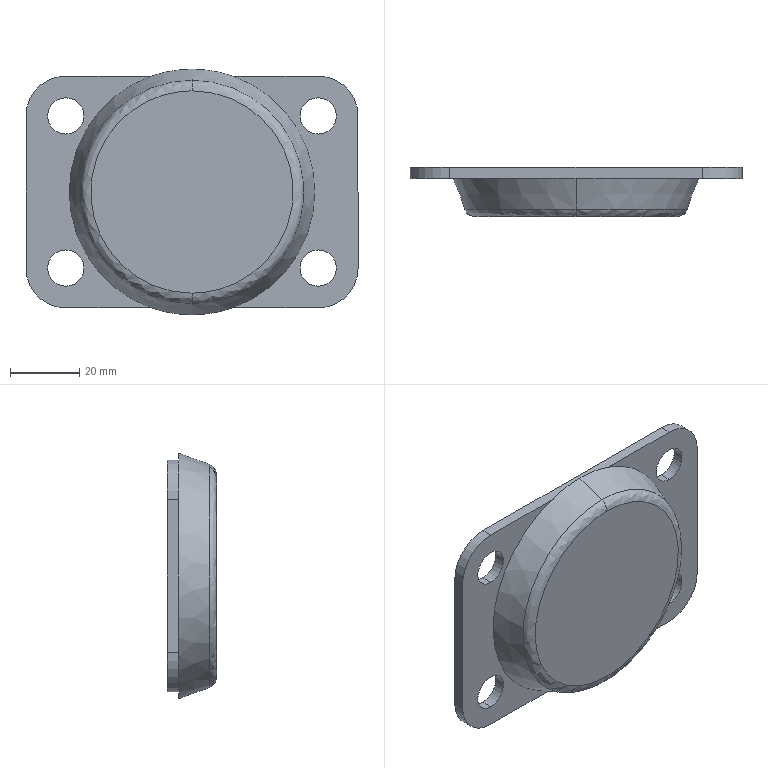Part | SolidWorks | features BaseBody 1 | 1 solid | 32 faces | box 96 x 14.2 x 71 mm | volume 54895 mm3 | cylinder 16 | plane 12 | spline 2 | cone 2 | commonest cylinder face diameters 10.5 x8 23 x4 27 x2 54 x2
STEP:
#1=CARTESIAN_POINT('',(0.,-12.094,-32.263));
#2=VERTEX_POINT('',#1);
#3=CARTESIAN_POINT('',(0.,-12.094,32.263));
#4=VERTEX_POINT('',#3);
#5=CARTESIAN_POINT('',(0.,-12.094,0.));
#6=DIRECTION('',(0.,1.,0.));
#7=DIRECTION('',(0.,0.,1.));
#8=AXIS2_PLACEMENT_3D('',#5,#6,#7);
#9=CIRCLE('',#8,32.263);
#10=EDGE_CURVE('',#2,#4,#9,.T.);
#11=ORIENTED_EDGE('',*,*,#10,.F.);
#12=CARTESIAN_POINT('',(0.,-14.2,-29.256));
#13=VERTEX_POINT('',#12);
#14=CARTESIAN_POINT('',(0.,-11.,-29.256));
#15=DIRECTION('',(-1.,0.,0.));
#16=DIRECTION('',(0.,0.,-1.));
#17=AXIS2_PLACEMENT_3D('',#14,#15,#16);
#18=CIRCLE('',#17,3.2);
#19=EDGE_CURVE('',#2,#13,#18,.T.);
#20=ORIENTED_EDGE('',*,*,#19,.T.);
#21=CARTESIAN_POINT('',(0.,-14.2,29.256));
#22=VERTEX_POINT('',#21);
#23=CARTESIAN_POINT('',(0.,-14.2,-29.256));
#24=CARTESIAN_POINT('',(-58.511,-14.2,-29.256));
#25=CARTESIAN_POINT('',(-58.511,-14.2,29.256));
#26=CARTESIAN_POINT('',(0.,-14.2,29.256));
#27=(BOUNDED_CURVE()B_SPLINE_CURVE(3,(#23,#24,#25,#26),.UNSPECIFIED.,.F.,.T.)B_SPLINE_CURVE_WITH_KNOTS((4,4),(0.,1.),.UNSPECIFIED.)CURVE()GEOMETRIC_REPRESENTATION_ITEM()RATIONAL_B_SPLINE_CURVE((1.,0.3333,0.3333,1.))REPRESENTATION_ITEM(''));
#28=EDGE_CURVE('',#13,#22,#27,.T.);
#29=ORIENTED_EDGE('',*,*,#28,.T.);
#30=CARTESIAN_POINT('',(0.,-11.,29.256));
#31=DIRECTION('',(1.,0.,0.));
#32=DIRECTION('',(0.,0.,1.));
#33=AXIS2_PLACEMENT_3D('',#30,#31,#32);
#34=CIRCLE('',#33,3.2);
#35=EDGE_CURVE('',#4,#22,#34,.T.);
#36=ORIENTED_EDGE('',*,*,#35,.F.);
#37=EDGE_LOOP('',(#11,#20,#29,#36));
#38=FACE_OUTER_BOUND('',#37,.T.);
#39=CARTESIAN_POINT('',(0.,-12.094,-32.263));
#40=CARTESIAN_POINT('',(-64.525,-12.094,-32.263));
#41=CARTESIAN_POINT('',(-64.525,-12.094,32.263));
#42=CARTESIAN_POINT('',(0.,-12.094,32.263));
#43=CARTESIAN_POINT('',(0.,-13.402,-31.787));
#44=CARTESIAN_POINT('',(-63.574,-13.402,-31.787));
#45=CARTESIAN_POINT('',(-63.574,-13.402,31.787));
#46=CARTESIAN_POINT('',(0.,-13.402,31.787));
#47=CARTESIAN_POINT('',(0.,-14.2,-30.647));
#48=CARTESIAN_POINT('',(-61.294,-14.2,-30.647));
#49=CARTESIAN_POINT('',(-61.294,-14.2,30.647));
#50=CARTESIAN_POINT('',(0.,-14.2,30.647));
#51=CARTESIAN_POINT('',(0.,-14.2,-29.256));
#52=CARTESIAN_POINT('',(-58.511,-14.2,-29.256));
#53=CARTESIAN_POINT('',(-58.511,-14.2,29.256));
#54=CARTESIAN_POINT('',(0.,-14.2,29.256));
#55=(BOUNDED_SURFACE()B_SPLINE_SURFACE(3,3,((#39,#40,#41,#42),(#43,#44,#45,#46),(#47,#48,#49,#50),(#51,#52,#53,#54)),.UNSPECIFIED.,.F.,.F.,.F.)B_SPLINE_SURFACE_WITH_KNOTS((4,4),(4,4),(0.,1.),(0.,1.),.UNSPECIFIED.)GEOMETRIC_REPRESENTATION_ITEM()RATIONAL_B_SPLINE_SURFACE(((1.,0.3333,0.3333,1.),(0.8794,0.2931,0.2931,0.8794),(0.8794,0.2931,0.2931,0.8794),(1.,0.3333,0.3333,1.)))REPRESENTATION_ITEM('')SURFACE());
#56=ADVANCED_FACE('',(#38),#55,.T.);
#57=CARTESIAN_POINT('',(36.5,-3.2,16.75));
#58=VERTEX_POINT('',#57);
#59=CARTESIAN_POINT('',(36.5,-3.2,27.25));
#60=VERTEX_POINT('',#59);
#61=CARTESIAN_POINT('',(36.5,-3.2,22.));
#62=DIRECTION('',(0.,1.,0.));
#63=DIRECTION('',(0.,0.,1.));
#64=AXIS2_PLACEMENT_3D('',#61,#62,#63);
#65=CIRCLE('',#64,5.25);
#66=EDGE_CURVE('',#58,#60,#65,.T.);
#67=ORIENTED_EDGE('',*,*,#66,.F.);
#68=CARTESIAN_POINT('',(36.5,0.,16.75));
#69=VERTEX_POINT('',#68);
#70=CARTESIAN_POINT('',(36.5,-3.2,16.75));
#71=DIRECTION('',(0.,1.,0.));
#72=VECTOR('',#71,1000.);
#73=LINE('',#70,#72);
#74=EDGE_CURVE('',#58,#69,#73,.T.);
#75=ORIENTED_EDGE('',*,*,#74,.T.);
#76=CARTESIAN_POINT('',(36.5,0.,27.25));
#77=VERTEX_POINT('',#76);
#78=CARTESIAN_POINT('',(36.5,0.,22.));
#79=DIRECTION('',(0.,-1.,0.));
#80=DIRECTION('',(0.,0.,1.));
#81=AXIS2_PLACEMENT_3D('',#78,#79,#80);
#82=CIRCLE('',#81,5.25);
#83=EDGE_CURVE('',#77,#69,#82,.T.);
#84=ORIENTED_EDGE('',*,*,#83,.F.);
#85=CARTESIAN_POINT('',(36.5,-3.2,27.25));
#86=DIRECTION('',(0.,1.,0.));
#87=VECTOR('',#86,1000.);
#88=LINE('',#85,#87);
#89=EDGE_CURVE('',#60,#77,#88,.T.);
#90=ORIENTED_EDGE('',*,*,#89,.F.);
#91=EDGE_LOOP('',(#67,#75,#84,#90));
#92=FACE_OUTER_BOUND('',#91,.T.);
#93=CARTESIAN_POINT('',(36.5,-3.2,22.));
#94=DIRECTION('',(0.,1.,0.));
#95=DIRECTION('',(0.,0.,1.));
#96=AXIS2_PLACEMENT_3D('',#93,#94,#95);
#97=CYLINDRICAL_SURFACE('',#96,5.25);
#98=ADVANCED_FACE('',(#92),#97,.F.);
#99=CARTESIAN_POINT('',(36.5,-3.2,-27.25));
#100=VERTEX_POINT('',#99);
#101=CARTESIAN_POINT('',(36.5,-3.2,-16.75));
#102=VERTEX_POINT('',#101);
#103=CARTESIAN_POINT('',(36.5,-3.2,-22.));
#104=DIRECTION('',(0.,1.,0.));
#105=DIRECTION('',(0.,0.,1.));
#106=AXIS2_PLACEMENT_3D('',#103,#104,#105);
#107=CIRCLE('',#106,5.25);
#108=EDGE_CURVE('',#100,#102,#107,.T.);
#109=ORIENTED_EDGE('',*,*,#108,.F.);
#110=CARTESIAN_POINT('',(36.5,0.,-27.25));
#111=VERTEX_POINT('',#110);
#112=CARTESIAN_POINT('',(36.5,-3.2,-27.25));
#113=DIRECTION('',(0.,1.,0.));
#114=VECTOR('',#113,1000.);
#115=LINE('',#112,#114);
#116=EDGE_CURVE('',#100,#111,#115,.T.);
#117=ORIENTED_EDGE('',*,*,#116,.T.);
#118=CARTESIAN_POINT('',(36.5,0.,-16.75));
#119=VERTEX_POINT('',#118);
#120=CARTESIAN_POINT('',(36.5,0.,-22.));
#121=DIRECTION('',(0.,-1.,0.));
#122=DIRECTION('',(0.,0.,1.));
#123=AXIS2_PLACEMENT_3D('',#120,#121,#122);
#124=CIRCLE('',#123,5.25);
#125=EDGE_CURVE('',#119,#111,#124,.T.);
#126=ORIENTED_EDGE('',*,*,#125,.F.);
#127=CARTESIAN_POINT('',(36.5,-3.2,-16.75));
#128=DIRECTION('',(0.,1.,0.));
#129=VECTOR('',#128,1000.);
#130=LINE('',#127,#129);
#131=EDGE_CURVE('',#102,#119,#130,.T.);
#132=ORIENTED_EDGE('',*,*,#131,.F.);
#133=EDGE_LOOP('',(#109,#117,#126,#132));
#134=FACE_OUTER_BOUND('',#133,.T.);
#135=CARTESIAN_POINT('',(36.5,-3.2,-22.));
#136=DIRECTION('',(0.,1.,0.));
#137=DIRECTION('',(0.,0.,1.));
#138=AXIS2_PLACEMENT_3D('',#135,#136,#137);
#139=CYLINDRICAL_SURFACE('',#138,5.25);
#140=ADVANCED_FACE('',(#134),#139,.F.);
#141=CARTESIAN_POINT('',(-36.5,-3.2,16.75));
#142=VERTEX_POINT('',#141);
#143=CARTESIAN_POINT('',(-36.5,-3.2,27.25));
#144=VERTEX_POINT('',#143);
#145=CARTESIAN_POINT('',(-36.5,-3.2,22.));
#146=DIRECTION('',(0.,1.,0.));
#147=DIRECTION('',(0.,0.,1.));
#148=AXIS2_PLACEMENT_3D('',#145,#146,#147);
#149=CIRCLE('',#148,5.25);
#150=EDGE_CURVE('',#142,#144,#149,.T.);
#151=ORIENTED_EDGE('',*,*,#150,.F.);
#152=CARTESIAN_POINT('',(-36.5,0.,16.75));
#153=VERTEX_POINT('',#152);
#154=CARTESIAN_POINT('',(-36.5,-3.2,16.75));
#155=DIRECTION('',(0.,1.,0.));
#156=VECTOR('',#155,1000.);
#157=LINE('',#154,#156);
#158=EDGE_CURVE('',#142,#153,#157,.T.);
#159=ORIENTED_EDGE('',*,*,#158,.T.);
#160=CARTESIAN_POINT('',(-36.5,0.,27.25));
#161=VERTEX_POINT('',#160);
#162=CARTESIAN_POINT('',(-36.5,0.,22.));
#163=DIRECTION('',(0.,-1.,0.));
#164=DIRECTION('',(0.,0.,1.));
#165=AXIS2_PLACEMENT_3D('',#162,#163,#164);
#166=CIRCLE('',#165,5.25);
#167=EDGE_CURVE('',#161,#153,#166,.T.);
#168=ORIENTED_EDGE('',*,*,#167,.F.);
#169=CARTESIAN_POINT('',(-36.5,-3.2,27.25));
#170=DIRECTION('',(0.,1.,0.));
#171=VECTOR('',#170,1000.);
#172=LINE('',#169,#171);
#173=EDGE_CURVE('',#144,#161,#172,.T.);
#174=ORIENTED_EDGE('',*,*,#173,.F.);
#175=EDGE_LOOP('',(#151,#159,#168,#174));
#176=FACE_OUTER_BOUND('',#175,.T.);
#177=CARTESIAN_POINT('',(-36.5,-3.2,22.));
#178=DIRECTION('',(0.,1.,0.));
#179=DIRECTION('',(0.,0.,1.));
#180=AXIS2_PLACEMENT_3D('',#177,#178,#179);
#181=CYLINDRICAL_SURFACE('',#180,5.25);
#182=ADVANCED_FACE('',(#176),#181,.F.);
#183=CARTESIAN_POINT('',(-36.5,-3.2,-27.25));
#184=VERTEX_POINT('',#183);
#185=CARTESIAN_POINT('',(-36.5,-3.2,-16.75));
#186=VERTEX_POINT('',#185);
#187=CARTESIAN_POINT('',(-36.5,-3.2,-22.));
#188=DIRECTION('',(0.,1.,0.));
#189=DIRECTION('',(0.,0.,1.));
#190=AXIS2_PLACEMENT_3D('',#187,#188,#189);
#191=CIRCLE('',#190,5.25);
#192=EDGE_CURVE('',#184,#186,#191,.T.);
#193=ORIENTED_EDGE('',*,*,#192,.F.);
#194=CARTESIAN_POINT('',(-36.5,0.,-27.25));
#195=VERTEX_POINT('',#194);
#196=CARTESIAN_POINT('',(-36.5,-3.2,-27.25));
#197=DIRECTION('',(0.,1.,0.));
#198=VECTOR('',#197,1000.);
#199=LINE('',#196,#198);
#200=EDGE_CURVE('',#184,#195,#199,.T.);
#201=ORIENTED_EDGE('',*,*,#200,.T.);
#202=CARTESIAN_POINT('',(-36.5,0.,-16.75));
#203=VERTEX_POINT('',#202);
#204=CARTESIAN_POINT('',(-36.5,0.,-22.));
#205=DIRECTION('',(0.,-1.,0.));
#206=DIRECTION('',(0.,0.,1.));
#207=AXIS2_PLACEMENT_3D('',#204,#205,#206);
#208=CIRCLE('',#207,5.25);
#209=EDGE_CURVE('',#203,#195,#208,.T.);
#210=ORIENTED_EDGE('',*,*,#209,.F.);
#211=CARTESIAN_POINT('',(-36.5,-3.2,-16.75));
#212=DIRECTION('',(0.,1.,0.));
#213=VECTOR('',#212,1000.);
#214=LINE('',#211,#213);
#215=EDGE_CURVE('',#186,#203,#214,.T.);
#216=ORIENTED_EDGE('',*,*,#215,.F.);
#217=EDGE_LOOP('',(#193,#201,#210,#216));
#218=FACE_OUTER_BOUND('',#217,.T.);
#219=CARTESIAN_POINT('',(-36.5,-3.2,-22.));
#220=DIRECTION('',(0.,1.,0.));
#221=DIRECTION('',(0.,0.,1.));
#222=AXIS2_PLACEMENT_3D('',#219,#220,#221);
#223=CYLINDRICAL_SURFACE('',#222,5.25);
#224=ADVANCED_FACE('',(#218),#223,.F.);
#225=CARTESIAN_POINT('',(0.,-1.5,-27.));
#226=VERTEX_POINT('',#225);
#227=CARTESIAN_POINT('',(0.,-1.5,27.));
#228=VERTEX_POINT('',#227);
#229=CARTESIAN_POINT('',(0.,-1.5,0.));
#230=DIRECTION('',(0.,1.,0.));
#231=DIRECTION('',(0.,0.,1.));
#232=AXIS2_PLACEMENT_3D('',#229,#230,#231);
#233=CIRCLE('',#232,27.);
#234=EDGE_CURVE('',#226,#228,#233,.T.);
#235=ORIENTED_EDGE('',*,*,#234,.F.);
#236=CARTESIAN_POINT('',(0.,0.,-27.));
#237=VERTEX_POINT('',#236);
#238=CARTESIAN_POINT('',(0.,-1.5,-27.));
#239=DIRECTION('',(0.,1.,0.));
#240=VECTOR('',#239,1000.);
#241=LINE('',#238,#240);
#242=EDGE_CURVE('',#226,#237,#241,.T.);
#243=ORIENTED_EDGE('',*,*,#242,.T.);
#244=CARTESIAN_POINT('',(0.,0.,27.));
#245=VERTEX_POINT('',#244);
#246=CARTESIAN_POINT('',(0.,0.,0.));
#247=DIRECTION('',(0.,-1.,0.));
#248=DIRECTION('',(0.,0.,1.));
#249=AXIS2_PLACEMENT_3D('',#246,#247,#248);
#250=CIRCLE('',#249,27.);
#251=EDGE_CURVE('',#245,#237,#250,.T.);
#252=ORIENTED_EDGE('',*,*,#251,.F.);
#253=CARTESIAN_POINT('',(0.,-1.5,27.));
#254=DIRECTION('',(0.,1.,0.));
#255=VECTOR('',#254,1000.);
#256=LINE('',#253,#255);
#257=EDGE_CURVE('',#228,#245,#256,.T.);
#258=ORIENTED_EDGE('',*,*,#257,.F.);
#259=EDGE_LOOP('',(#235,#243,#252,#258));
#260=FACE_OUTER_BOUND('',#259,.T.);
#261=CARTESIAN_POINT('',(0.,-1.5,0.));
#262=DIRECTION('',(0.,1.,0.));
#263=DIRECTION('',(0.,0.,1.));
#264=AXIS2_PLACEMENT_3D('',#261,#262,#263);
#265=CYLINDRICAL_SURFACE('',#264,27.);
#266=ADVANCED_FACE('',(#260),#265,.F.);
#267=CARTESIAN_POINT('',(0.,-12.094,0.));
#268=DIRECTION('',(0.,1.,0.));
#269=DIRECTION('',(0.,0.,1.));
#270=AXIS2_PLACEMENT_3D('',#267,#268,#269);
#271=CIRCLE('',#270,32.263);
#272=EDGE_CURVE('',#4,#2,#271,.T.);
#273=ORIENTED_EDGE('',*,*,#272,.T.);
#274=CARTESIAN_POINT('',(0.,-3.2,-35.5));
#275=VERTEX_POINT('',#274);
#276=CARTESIAN_POINT('',(0.,-3.2,-35.5));
#277=DIRECTION('',(0.,0.9397,-0.342));
#278=VECTOR('',#277,1000.);
#279=LINE('',#276,#278);
#280=EDGE_CURVE('',#2,#275,#279,.T.);
#281=ORIENTED_EDGE('',*,*,#280,.T.);
#282=CARTESIAN_POINT('',(11.747,-3.2,-33.5));
#283=VERTEX_POINT('',#282);
#284=CARTESIAN_POINT('',(0.,-3.2,0.));
#285=DIRECTION('',(0.,1.,0.));
#286=DIRECTION('',(0.,0.,1.));
#287=AXIS2_PLACEMENT_3D('',#284,#285,#286);
#288=CIRCLE('',#287,35.5);
#289=EDGE_CURVE('',#283,#275,#288,.T.);
#290=ORIENTED_EDGE('',*,*,#289,.F.);
#291=CARTESIAN_POINT('',(11.747,-3.2,33.5));
#292=VERTEX_POINT('',#291);
#293=CARTESIAN_POINT('',(0.,-3.2,0.));
#294=DIRECTION('',(0.,-1.,0.));
#295=DIRECTION('',(0.,0.,1.));
#296=AXIS2_PLACEMENT_3D('',#293,#294,#295);
#297=CIRCLE('',#296,35.5);
#298=EDGE_CURVE('',#283,#292,#297,.T.);
#299=ORIENTED_EDGE('',*,*,#298,.T.);
#300=CARTESIAN_POINT('',(0.,-3.2,35.5));
#301=VERTEX_POINT('',#300);
#302=CARTESIAN_POINT('',(0.,-3.2,0.));
#303=DIRECTION('',(0.,1.,0.));
#304=DIRECTION('',(0.,0.,1.));
#305=AXIS2_PLACEMENT_3D('',#302,#303,#304);
#306=CIRCLE('',#305,35.5);
#307=EDGE_CURVE('',#301,#292,#306,.T.);
#308=ORIENTED_EDGE('',*,*,#307,.F.);
#309=CARTESIAN_POINT('',(0.,-3.2,35.5));
#310=DIRECTION('',(0.,0.9397,0.342));
#311=VECTOR('',#310,1000.);
#312=LINE('',#309,#311);
#313=EDGE_CURVE('',#4,#301,#312,.T.);
#314=ORIENTED_EDGE('',*,*,#313,.F.);
#315=EDGE_LOOP('',(#273,#281,#290,#299,#308,#314));
#316=FACE_OUTER_BOUND('',#315,.T.);
#317=CARTESIAN_POINT('',(0.,-3.2,0.));
#318=DIRECTION('',(0.,1.,0.));
#319=DIRECTION('',(0.,0.,1.));
#320=AXIS2_PLACEMENT_3D('',#317,#318,#319);
#321=CONICAL_SURFACE('',#320,35.5,0.3491);
#322=ADVANCED_FACE('',(#316),#321,.T.);
#323=CARTESIAN_POINT('',(0.,-0.5,-13.5));
#324=VERTEX_POINT('',#323);
#325=CARTESIAN_POINT('',(0.,-0.5,13.5));
#326=VERTEX_POINT('',#325);
#327=CARTESIAN_POINT('',(0.,-0.5,0.));
#328=DIRECTION('',(0.,-1.,0.));
#329=DIRECTION('',(0.,0.,-1.));
#330=AXIS2_PLACEMENT_3D('',#327,#328,#329);
#331=CIRCLE('',#330,13.5);
#332=EDGE_CURVE('',#324,#326,#331,.T.);
#333=ORIENTED_EDGE('',*,*,#332,.T.);
#334=CARTESIAN_POINT('',(0.,-1.5,13.5));
#335=VERTEX_POINT('',#334);
#336=CARTESIAN_POINT('',(0.,-0.5,13.5));
#337=DIRECTION('',(0.,-1.,0.));
#338=VECTOR('',#337,1000.);
#339=LINE('',#336,#338);
#340=EDGE_CURVE('',#326,#335,#339,.T.);
#341=ORIENTED_EDGE('',*,*,#340,.T.);
#342=CARTESIAN_POINT('',(0.,-1.5,-13.5));
#343=VERTEX_POINT('',#342);
#344=CARTESIAN_POINT('',(0.,-1.5,0.));
#345=DIRECTION('',(0.,-1.,0.));
#346=DIRECTION('',(0.,0.,-1.));
#347=AXIS2_PLACEMENT_3D('',#344,#345,#346);
#348=CIRCLE('',#347,13.5);
#349=EDGE_CURVE('',#343,#335,#348,.T.);
#350=ORIENTED_EDGE('',*,*,#349,.F.);
#351=CARTESIAN_POINT('',(0.,-0.5,-13.5));
#352=DIRECTION('',(0.,-1.,0.));
#353=VECTOR('',#352,1000.);
#354=LINE('',#351,#353);
#355=EDGE_CURVE('',#324,#343,#354,.T.);
#356=ORIENTED_EDGE('',*,*,#355,.F.);
#357=EDGE_LOOP('',(#333,#341,#350,#356));
#358=FACE_OUTER_BOUND('',#357,.T.);
#359=CARTESIAN_POINT('',(0.,-0.5,0.));
#360=DIRECTION('',(0.,-1.,0.));
#361=DIRECTION('',(0.,0.,-1.));
#362=AXIS2_PLACEMENT_3D('',#359,#360,#361);
#363=CYLINDRICAL_SURFACE('',#362,13.5);
#364=ADVANCED_FACE('',(#358),#363,.T.);
#365=CARTESIAN_POINT('',(-36.5,0.,-33.5));
#366=VERTEX_POINT('',#365);
#367=CARTESIAN_POINT('',(-48.,0.,-22.));
#368=VERTEX_POINT('',#367);
#369=CARTESIAN_POINT('',(-36.5,0.,-22.));
#370=DIRECTION('',(0.,1.,0.));
#371=DIRECTION('',(0.,0.,1.));
#372=AXIS2_PLACEMENT_3D('',#369,#370,#371);
#373=CIRCLE('',#372,11.5);
#374=EDGE_CURVE('',#366,#368,#373,.T.);
#375=ORIENTED_EDGE('',*,*,#374,.T.);
#376=CARTESIAN_POINT('',(-48.,0.,22.));
#377=VERTEX_POINT('',#376);
#378=CARTESIAN_POINT('',(-48.,0.,22.));
#379=DIRECTION('',(0.,0.,1.));
#380=VECTOR('',#379,1000.);
#381=LINE('',#378,#380);
#382=EDGE_CURVE('',#368,#377,#381,.T.);
#383=ORIENTED_EDGE('',*,*,#382,.T.);
#384=CARTESIAN_POINT('',(-36.5,0.,33.5));
#385=VERTEX_POINT('',#384);
#386=CARTESIAN_POINT('',(-36.5,0.,22.));
#387=DIRECTION('',(0.,1.,0.));
#388=DIRECTION('',(0.,0.,1.));
#389=AXIS2_PLACEMENT_3D('',#386,#387,#388);
#390=CIRCLE('',#389,11.5);
#391=EDGE_CURVE('',#377,#385,#390,.T.);
#392=ORIENTED_EDGE('',*,*,#391,.T.);
#393=CARTESIAN_POINT('',(36.5,0.,33.5));
#394=VERTEX_POINT('',#393);
#395=CARTESIAN_POINT('',(-36.5,0.,33.5));
#396=DIRECTION('',(1.,0.,0.));
#397=VECTOR('',#396,1000.);
#398=LINE('',#395,#397);
#399=EDGE_CURVE('',#385,#394,#398,.T.);
#400=ORIENTED_EDGE('',*,*,#399,.T.);
#401=CARTESIAN_POINT('',(48.,0.,22.));
#402=VERTEX_POINT('',#401);
#403=CARTESIAN_POINT('',(36.5,0.,22.));
#404=DIRECTION('',(0.,1.,0.));
#405=DIRECTION('',(0.,0.,1.));
#406=AXIS2_PLACEMENT_3D('',#403,#404,#405);
#407=CIRCLE('',#406,11.5);
#408=EDGE_CURVE('',#394,#402,#407,.T.);
#409=ORIENTED_EDGE('',*,*,#408,.T.);
#410=CARTESIAN_POINT('',(48.,0.,-22.));
#411=VERTEX_POINT('',#410);
#412=CARTESIAN_POINT('',(48.,0.,22.));
#413=DIRECTION('',(0.,0.,-1.));
#414=VECTOR('',#413,1000.);
#415=LINE('',#412,#414);
#416=EDGE_CURVE('',#402,#411,#415,.T.);
#417=ORIENTED_EDGE('',*,*,#416,.T.);
#418=CARTESIAN_POINT('',(36.5,0.,-33.5));
#419=VERTEX_POINT('',#418);
#420=CARTESIAN_POINT('',(36.5,0.,-22.));
#421=DIRECTION('',(0.,1.,0.));
#422=DIRECTION('',(0.,0.,1.));
#423=AXIS2_PLACEMENT_3D('',#420,#421,#422);
#424=CIRCLE('',#423,11.5);
#425=EDGE_CURVE('',#411,#419,#424,.T.);
#426=ORIENTED_EDGE('',*,*,#425,.T.);
#427=CARTESIAN_POINT('',(-36.5,0.,-33.5));
#428=DIRECTION('',(-1.,0.,0.));
#429=VECTOR('',#428,1000.);
#430=LINE('',#427,#429);
#431=EDGE_CURVE('',#419,#366,#430,.T.);
#432=ORIENTED_EDGE('',*,*,#431,.T.);
#433=EDGE_LOOP('',(#375,#383,#392,#400,#409,#417,#426,#432));
#434=FACE_OUTER_BOUND('',#433,.T.);
#435=ORIENTED_EDGE('',*,*,#83,.T.);
#436=CARTESIAN_POINT('',(36.5,0.,22.));
#437=DIRECTION('',(0.,-1.,0.));
#438=DIRECTION('',(0.,0.,1.));
#439=AXIS2_PLACEMENT_3D('',#436,#437,#438);
#440=CIRCLE('',#439,5.25);
#441=EDGE_CURVE('',#69,#77,#440,.T.);
#442=ORIENTED_EDGE('',*,*,#441,.T.);
#443=EDGE_LOOP('',(#435,#442));
#444=FACE_BOUND('',#443,.T.);
#445=ORIENTED_EDGE('',*,*,#125,.T.);
#446=CARTESIAN_POINT('',(36.5,0.,-22.));
#447=DIRECTION('',(0.,-1.,0.));
#448=DIRECTION('',(0.,0.,1.));
#449=AXIS2_PLACEMENT_3D('',#446,#447,#448);
#450=CIRCLE('',#449,5.25);
#451=EDGE_CURVE('',#111,#119,#450,.T.);
#452=ORIENTED_EDGE('',*,*,#451,.T.);
#453=EDGE_LOOP('',(#445,#452));
#454=FACE_BOUND('',#453,.T.);
#455=ORIENTED_EDGE('',*,*,#167,.T.);
#456=CARTESIAN_POINT('',(-36.5,0.,22.));
#457=DIRECTION('',(0.,-1.,0.));
#458=DIRECTION('',(0.,0.,1.));
#459=AXIS2_PLACEMENT_3D('',#456,#457,#458);
#460=CIRCLE('',#459,5.25);
#461=EDGE_CURVE('',#153,#161,#460,.T.);
#462=ORIENTED_EDGE('',*,*,#461,.T.);
#463=EDGE_LOOP('',(#455,#462));
#464=FACE_BOUND('',#463,.T.);
#465=ORIENTED_EDGE('',*,*,#209,.T.);
#466=CARTESIAN_POINT('',(-36.5,0.,-22.));
#467=DIRECTION('',(0.,-1.,0.));
#468=DIRECTION('',(0.,0.,1.));
#469=AXIS2_PLACEMENT_3D('',#466,#467,#468);
#470=CIRCLE('',#469,5.25);
#471=EDGE_CURVE('',#195,#203,#470,.T.);
#472=ORIENTED_EDGE('',*,*,#471,.T.);
#473=EDGE_LOOP('',(#465,#472));
#474=FACE_BOUND('',#473,.T.);
#475=ORIENTED_EDGE('',*,*,#251,.T.);
#476=CARTESIAN_POINT('',(0.,0.,0.));
#477=DIRECTION('',(0.,-1.,0.));
#478=DIRECTION('',(0.,0.,1.));
#479=AXIS2_PLACEMENT_3D('',#476,#477,#478);
#480=CIRCLE('',#479,27.);
#481=EDGE_CURVE('',#237,#245,#480,.T.);
#482=ORIENTED_EDGE('',*,*,#481,.T.);
#483=EDGE_LOOP('',(#475,#482));
#484=FACE_BOUND('',#483,.T.);
#485=CARTESIAN_POINT('',(-36.5,0.,22.));
#486=DIRECTION('',(0.,1.,0.));
#487=DIRECTION('',(0.,0.,1.));
#488=AXIS2_PLACEMENT_3D('',#485,#486,#487);
#489=PLANE('',#488);
#490=ADVANCED_FACE('',(#434,#444,#454,#464,#474,#484),#489,.T.);
#491=CARTESIAN_POINT('',(-48.,-3.2,-22.));
#492=VERTEX_POINT('',#491);
#493=CARTESIAN_POINT('',(-48.,-3.2,22.));
#494=VERTEX_POINT('',#493);
#495=CARTESIAN_POINT('',(-48.,-3.2,-22.));
#496=DIRECTION('',(0.,0.,1.));
#497=VECTOR('',#496,1000.);
#498=LINE('',#495,#497);
#499=EDGE_CURVE('',#492,#494,#498,.T.);
#500=ORIENTED_EDGE('',*,*,#499,.T.);
#501=CARTESIAN_POINT('',(-48.,-3.2,22.));
#502=DIRECTION('',(0.,1.,0.));
#503=VECTOR('',#502,1000.);
#504=LINE('',#501,#503);
#505=EDGE_CURVE('',#494,#377,#504,.T.);
#506=ORIENTED_EDGE('',*,*,#505,.T.);
#507=ORIENTED_EDGE('',*,*,#382,.F.);
#508=CARTESIAN_POINT('',(-48.,-3.2,-22.));
#509=DIRECTION('',(0.,-1.,0.));
#510=VECTOR('',#509,1000.);
#511=LINE('',#508,#510);
#512=EDGE_CURVE('',#368,#492,#511,.T.);
#513=ORIENTED_EDGE('',*,*,#512,.T.);
#514=EDGE_LOOP('',(#500,#506,#507,#513));
#515=FACE_OUTER_BOUND('',#514,.T.);
#516=CARTESIAN_POINT('',(-48.,-3.2,-22.));
#517=DIRECTION('',(-1.,0.,0.));
#518=DIRECTION('',(0.,0.,1.));
#519=AXIS2_PLACEMENT_3D('',#516,#517,#518);
#520=PLANE('',#519);
#521=ADVANCED_FACE('',(#515),#520,.T.);
#522=CARTESIAN_POINT('',(-36.5,-3.2,-33.5));
#523=VERTEX_POINT('',#522);
#524=CARTESIAN_POINT('',(-36.5,-3.2,-22.));
#525=DIRECTION('',(0.,1.,0.));
#526=DIRECTION('',(0.,0.,1.));
#527=AXIS2_PLACEMENT_3D('',#524,#525,#526);
#528=CIRCLE('',#527,11.5);
#529=EDGE_CURVE('',#523,#492,#528,.T.);
#530=ORIENTED_EDGE('',*,*,#529,.T.);
#531=ORIENTED_EDGE('',*,*,#512,.F.);
#532=ORIENTED_EDGE('',*,*,#374,.F.);
#533=CARTESIAN_POINT('',(-36.5,-3.2,-33.5));
#534=DIRECTION('',(0.,-1.,0.));
#535=VECTOR('',#534,1000.);
#536=LINE('',#533,#535);
#537=EDGE_CURVE('',#366,#523,#536,.T.);
#538=ORIENTED_EDGE('',*,*,#537,.T.);
#539=EDGE_LOOP('',(#530,#531,#532,#538));
#540=FACE_OUTER_BOUND('',#539,.T.);
#541=CARTESIAN_POINT('',(-36.5,-3.2,-22.));
#542=DIRECTION('',(0.,1.,0.));
#543=DIRECTION('',(0.,0.,1.));
#544=AXIS2_PLACEMENT_3D('',#541,#542,#543);
#545=CYLINDRICAL_SURFACE('',#544,11.5);
#546=ADVANCED_FACE('',(#540),#545,.T.);
#547=CARTESIAN_POINT('',(-11.747,-3.2,-33.5));
#548=VERTEX_POINT('',#547);
#549=CARTESIAN_POINT('',(36.5,-3.2,-33.5));
#550=DIRECTION('',(-1.,0.,0.));
#551=VECTOR('',#550,1000.);
#552=LINE('',#549,#551);
#553=EDGE_CURVE('',#548,#523,#552,.T.);
#554=ORIENTED_EDGE('',*,*,#553,.T.);
#555=ORIENTED_EDGE('',*,*,#537,.F.);
#556=ORIENTED_EDGE('',*,*,#431,.F.);
#557=CARTESIAN_POINT('',(36.5,-3.2,-33.5));
#558=VERTEX_POINT('',#557);
#559=CARTESIAN_POINT('',(36.5,-3.2,-33.5));
#560=DIRECTION('',(0.,-1.,0.));
#561=VECTOR('',#560,1000.);
#562=LINE('',#559,#561);
#563=EDGE_CURVE('',#419,#558,#562,.T.);
#564=ORIENTED_EDGE('',*,*,#563,.T.);
#565=CARTESIAN_POINT('',(36.5,-3.2,-33.5));
#566=DIRECTION('',(-1.,0.,0.));
#567=VECTOR('',#566,1000.);
#568=LINE('',#565,#567);
#569=EDGE_CURVE('',#558,#283,#568,.T.);
#570=ORIENTED_EDGE('',*,*,#569,.T.);
#571=CARTESIAN_POINT('',(36.5,-3.2,-33.5));
#572=DIRECTION('',(-1.,0.,0.));
#573=VECTOR('',#572,1000.);
#574=LINE('',#571,#573);
#575=EDGE_CURVE('',#283,#548,#574,.T.);
#576=ORIENTED_EDGE('',*,*,#575,.T.);
#577=EDGE_LOOP('',(#554,#555,#556,#564,#570,#576));
#578=FACE_OUTER_BOUND('',#577,.T.);
#579=CARTESIAN_POINT('',(36.5,-3.2,-33.5));
#580=DIRECTION('',(0.,0.,-1.));
#581=DIRECTION('',(-1.,0.,0.));
#582=AXIS2_PLACEMENT_3D('',#579,#580,#581);
#583=PLANE('',#582);
#584=ADVANCED_FACE('',(#578),#583,.T.);
#585=CARTESIAN_POINT('',(48.,-3.2,-22.));
#586=VERTEX_POINT('',#585);
#587=CARTESIAN_POINT('',(36.5,-3.2,-22.));
#588=DIRECTION('',(0.,1.,0.));
#589=DIRECTION('',(0.,0.,1.));
#590=AXIS2_PLACEMENT_3D('',#587,#588,#589);
#591=CIRCLE('',#590,11.5);
#592=EDGE_CURVE('',#586,#558,#591,.T.);
#593=ORIENTED_EDGE('',*,*,#592,.T.);
#594=ORIENTED_EDGE('',*,*,#563,.F.);
#595=ORIENTED_EDGE('',*,*,#425,.F.);
#596=CARTESIAN_POINT('',(48.,-3.2,-22.));
#597=DIRECTION('',(0.,-1.,0.));
#598=VECTOR('',#597,1000.);
#599=LINE('',#596,#598);
#600=EDGE_CURVE('',#411,#586,#599,.T.);
#601=ORIENTED_EDGE('',*,*,#600,.T.);
#602=EDGE_LOOP('',(#593,#594,#595,#601));
#603=FACE_OUTER_BOUND('',#602,.T.);
#604=CARTESIAN_POINT('',(36.5,-3.2,-22.));
#605=DIRECTION('',(0.,1.,0.));
#606=DIRECTION('',(0.,0.,1.));
#607=AXIS2_PLACEMENT_3D('',#604,#605,#606);
#608=CYLINDRICAL_SURFACE('',#607,11.5);
#609=ADVANCED_FACE('',(#603),#608,.T.);
#610=CARTESIAN_POINT('',(48.,-3.2,22.));
#611=VERTEX_POINT('',#610);
#612=CARTESIAN_POINT('',(48.,-3.2,22.));
#613=DIRECTION('',(0.,0.,-1.));
#614=VECTOR('',#613,1000.);
#615=LINE('',#612,#614);
#616=EDGE_CURVE('',#611,#586,#615,.T.);
#617=ORIENTED_EDGE('',*,*,#616,.T.);
#618=ORIENTED_EDGE('',*,*,#600,.F.);
#619=ORIENTED_EDGE('',*,*,#416,.F.);
#620=CARTESIAN_POINT('',(48.,-3.2,22.));
#621=DIRECTION('',(0.,-1.,0.));
#622=VECTOR('',#621,1000.);
#623=LINE('',#620,#622);
#624=EDGE_CURVE('',#402,#611,#623,.T.);
#625=ORIENTED_EDGE('',*,*,#624,.T.);
#626=EDGE_LOOP('',(#617,#618,#619,#625));
#627=FACE_OUTER_BOUND('',#626,.T.);
#628=CARTESIAN_POINT('',(48.,-3.2,22.));
#629=DIRECTION('',(1.,0.,0.));
#630=DIRECTION('',(0.,0.,-1.));
#631=AXIS2_PLACEMENT_3D('',#628,#629,#630);
#632=PLANE('',#631);
#633=ADVANCED_FACE('',(#627),#632,.T.);
#634=CARTESIAN_POINT('',(36.5,-3.2,33.5));
#635=VERTEX_POINT('',#634);
#636=CARTESIAN_POINT('',(36.5,-3.2,22.));
#637=DIRECTION('',(0.,1.,0.));
#638=DIRECTION('',(0.,0.,1.));
#639=AXIS2_PLACEMENT_3D('',#636,#637,#638);
#640=CIRCLE('',#639,11.5);
#641=EDGE_CURVE('',#635,#611,#640,.T.);
#642=ORIENTED_EDGE('',*,*,#641,.T.);
#643=ORIENTED_EDGE('',*,*,#624,.F.);
#644=ORIENTED_EDGE('',*,*,#408,.F.);
#645=CARTESIAN_POINT('',(36.5,-3.2,33.5));
#646=DIRECTION('',(0.,-1.,0.));
#647=VECTOR('',#646,1000.);
#648=LINE('',#645,#647);
#649=EDGE_CURVE('',#394,#635,#648,.T.);
#650=ORIENTED_EDGE('',*,*,#649,.T.);
#651=EDGE_LOOP('',(#642,#643,#644,#650));
#652=FACE_OUTER_BOUND('',#651,.T.);
#653=CARTESIAN_POINT('',(36.5,-3.2,22.));
#654=DIRECTION('',(0.,1.,0.));
#655=DIRECTION('',(0.,0.,1.));
#656=AXIS2_PLACEMENT_3D('',#653,#654,#655);
#657=CYLINDRICAL_SURFACE('',#656,11.5);
#658=ADVANCED_FACE('',(#652),#657,.T.);
#659=CARTESIAN_POINT('',(-36.5,-3.2,33.5));
#660=DIRECTION('',(1.,0.,0.));
#661=VECTOR('',#660,1000.);
#662=LINE('',#659,#661);
#663=EDGE_CURVE('',#292,#635,#662,.T.);
#664=ORIENTED_EDGE('',*,*,#663,.T.);
#665=ORIENTED_EDGE('',*,*,#649,.F.);
#666=ORIENTED_EDGE('',*,*,#399,.F.);
#667=CARTESIAN_POINT('',(-36.5,-3.2,33.5));
#668=VERTEX_POINT('',#667);
#669=CARTESIAN_POINT('',(-36.5,-3.2,33.5));
#670=DIRECTION('',(0.,-1.,0.));
#671=VECTOR('',#670,1000.);
#672=LINE('',#669,#671);
#673=EDGE_CURVE('',#385,#668,#672,.T.);
#674=ORIENTED_EDGE('',*,*,#673,.T.);
#675=CARTESIAN_POINT('',(-11.747,-3.2,33.5));
#676=VERTEX_POINT('',#675);
#677=CARTESIAN_POINT('',(-36.5,-3.2,33.5));
#678=DIRECTION('',(1.,0.,0.));
#679=VECTOR('',#678,1000.);
#680=LINE('',#677,#679);
#681=EDGE_CURVE('',#668,#676,#680,.T.);
#682=ORIENTED_EDGE('',*,*,#681,.T.);
#683=CARTESIAN_POINT('',(-36.5,-3.2,33.5));
#684=DIRECTION('',(1.,0.,0.));
#685=VECTOR('',#684,1000.);
#686=LINE('',#683,#685);
#687=EDGE_CURVE('',#676,#292,#686,.T.);
#688=ORIENTED_EDGE('',*,*,#687,.T.);
#689=EDGE_LOOP('',(#664,#665,#666,#674,#682,#688));
#690=FACE_OUTER_BOUND('',#689,.T.);
#691=CARTESIAN_POINT('',(-36.5,-3.2,33.5));
#692=DIRECTION('',(0.,0.,1.));
#693=DIRECTION('',(1.,0.,0.));
#694=AXIS2_PLACEMENT_3D('',#691,#692,#693);
#695=PLANE('',#694);
#696=ADVANCED_FACE('',(#690),#695,.T.);
#697=CARTESIAN_POINT('',(-36.5,-3.2,22.));
#698=DIRECTION('',(0.,1.,0.));
#699=DIRECTION('',(0.,0.,1.));
#700=AXIS2_PLACEMENT_3D('',#697,#698,#699);
#701=CIRCLE('',#700,11.5);
#702=EDGE_CURVE('',#494,#668,#701,.T.);
#703=ORIENTED_EDGE('',*,*,#702,.T.);
#704=ORIENTED_EDGE('',*,*,#673,.F.);
#705=ORIENTED_EDGE('',*,*,#391,.F.);
#706=ORIENTED_EDGE('',*,*,#505,.F.);
#707=EDGE_LOOP('',(#703,#704,#705,#706));
#708=FACE_OUTER_BOUND('',#707,.T.);
#709=CARTESIAN_POINT('',(-36.5,-3.2,22.));
#710=DIRECTION('',(0.,1.,0.));
#711=DIRECTION('',(0.,0.,1.));
#712=AXIS2_PLACEMENT_3D('',#709,#710,#711);
#713=CYLINDRICAL_SURFACE('',#712,11.5);
#714=ADVANCED_FACE('',(#708),#713,.T.);
#715=ORIENTED_EDGE('',*,*,#74,.F.);
#716=CARTESIAN_POINT('',(36.5,-3.2,22.));
#717=DIRECTION('',(0.,1.,0.));
#718=DIRECTION('',(0.,0.,1.));
#719=AXIS2_PLACEMENT_3D('',#716,#717,#718);
#720=CIRCLE('',#719,5.25);
#721=EDGE_CURVE('',#60,#58,#720,.T.);
#722=ORIENTED_EDGE('',*,*,#721,.F.);
#723=ORIENTED_EDGE('',*,*,#89,.T.);
#724=ORIENTED_EDGE('',*,*,#441,.F.);
#725=EDGE_LOOP('',(#715,#722,#723,#724));
#726=FACE_OUTER_BOUND('',#725,.T.);
#727=CARTESIAN_POINT('',(36.5,-3.2,22.));
#728=DIRECTION('',(0.,1.,0.));
#729=DIRECTION('',(0.,0.,1.));
#730=AXIS2_PLACEMENT_3D('',#727,#728,#729);
#731=CYLINDRICAL_SURFACE('',#730,5.25);
#732=ADVANCED_FACE('',(#726),#731,.F.);
#733=ORIENTED_EDGE('',*,*,#116,.F.);
#734=CARTESIAN_POINT('',(36.5,-3.2,-22.));
#735=DIRECTION('',(0.,1.,0.));
#736=DIRECTION('',(0.,0.,1.));
#737=AXIS2_PLACEMENT_3D('',#734,#735,#736);
#738=CIRCLE('',#737,5.25);
#739=EDGE_CURVE('',#102,#100,#738,.T.);
#740=ORIENTED_EDGE('',*,*,#739,.F.);
#741=ORIENTED_EDGE('',*,*,#131,.T.);
#742=ORIENTED_EDGE('',*,*,#451,.F.);
#743=EDGE_LOOP('',(#733,#740,#741,#742));
#744=FACE_OUTER_BOUND('',#743,.T.);
#745=CARTESIAN_POINT('',(36.5,-3.2,-22.));
#746=DIRECTION('',(0.,1.,0.));
#747=DIRECTION('',(0.,0.,1.));
#748=AXIS2_PLACEMENT_3D('',#745,#746,#747);
#749=CYLINDRICAL_SURFACE('',#748,5.25);
#750=ADVANCED_FACE('',(#744),#749,.F.);
#751=ORIENTED_EDGE('',*,*,#158,.F.);
#752=CARTESIAN_POINT('',(-36.5,-3.2,22.));
#753=DIRECTION('',(0.,1.,0.));
#754=DIRECTION('',(0.,0.,1.));
#755=AXIS2_PLACEMENT_3D('',#752,#753,#754);
#756=CIRCLE('',#755,5.25);
#757=EDGE_CURVE('',#144,#142,#756,.T.);
#758=ORIENTED_EDGE('',*,*,#757,.F.);
#759=ORIENTED_EDGE('',*,*,#173,.T.);
#760=ORIENTED_EDGE('',*,*,#461,.F.);
#761=EDGE_LOOP('',(#751,#758,#759,#760));
#762=FACE_OUTER_BOUND('',#761,.T.);
#763=CARTESIAN_POINT('',(-36.5,-3.2,22.));
#764=DIRECTION('',(0.,1.,0.));
#765=DIRECTION('',(0.,0.,1.));
#766=AXIS2_PLACEMENT_3D('',#763,#764,#765);
#767=CYLINDRICAL_SURFACE('',#766,5.25);
#768=ADVANCED_FACE('',(#762),#767,.F.);
#769=ORIENTED_EDGE('',*,*,#200,.F.);
#770=CARTESIAN_POINT('',(-36.5,-3.2,-22.));
#771=DIRECTION('',(0.,1.,0.));
#772=DIRECTION('',(0.,0.,1.));
#773=AXIS2_PLACEMENT_3D('',#770,#771,#772);
#774=CIRCLE('',#773,5.25);
#775=EDGE_CURVE('',#186,#184,#774,.T.);
#776=ORIENTED_EDGE('',*,*,#775,.F.);
#777=ORIENTED_EDGE('',*,*,#215,.T.);
#778=ORIENTED_EDGE('',*,*,#471,.F.);
#779=EDGE_LOOP('',(#769,#776,#777,#778));
#780=FACE_OUTER_BOUND('',#779,.T.);
#781=CARTESIAN_POINT('',(-36.5,-3.2,-22.));
#782=DIRECTION('',(0.,1.,0.));
#783=DIRECTION('',(0.,0.,1.));
#784=AXIS2_PLACEMENT_3D('',#781,#782,#783);
#785=CYLINDRICAL_SURFACE('',#784,5.25);
#786=ADVANCED_FACE('',(#780),#785,.F.);
#787=ORIENTED_EDGE('',*,*,#242,.F.);
#788=CARTESIAN_POINT('',(0.,-1.5,0.));
#789=DIRECTION('',(0.,1.,0.));
#790=DIRECTION('',(0.,0.,1.));
#791=AXIS2_PLACEMENT_3D('',#788,#789,#790);
#792=CIRCLE('',#791,27.);
#793=EDGE_CURVE('',#228,#226,#792,.T.);
#794=ORIENTED_EDGE('',*,*,#793,.F.);
#795=ORIENTED_EDGE('',*,*,#257,.T.);
#796=ORIENTED_EDGE('',*,*,#481,.F.);
#797=EDGE_LOOP('',(#787,#794,#795,#796));
#798=FACE_OUTER_BOUND('',#797,.T.);
#799=CARTESIAN_POINT('',(0.,-1.5,0.));
#800=DIRECTION('',(0.,1.,0.));
#801=DIRECTION('',(0.,0.,1.));
#802=AXIS2_PLACEMENT_3D('',#799,#800,#801);
#803=CYLINDRICAL_SURFACE('',#802,27.);
#804=ADVANCED_FACE('',(#798),#803,.F.);
#805=CARTESIAN_POINT('',(0.,-3.2,0.));
#806=DIRECTION('',(0.,-1.,0.));
#807=DIRECTION('',(0.,0.,1.));
#808=AXIS2_PLACEMENT_3D('',#805,#806,#807);
#809=CIRCLE('',#808,35.5);
#810=EDGE_CURVE('',#676,#548,#809,.T.);
#811=ORIENTED_EDGE('',*,*,#810,.F.);
#812=ORIENTED_EDGE('',*,*,#681,.F.);
#813=ORIENTED_EDGE('',*,*,#702,.F.);
#814=ORIENTED_EDGE('',*,*,#499,.F.);
#815=ORIENTED_EDGE('',*,*,#529,.F.);
#816=ORIENTED_EDGE('',*,*,#553,.F.);
#817=EDGE_LOOP('',(#811,#812,#813,#814,#815,#816));
#818=FACE_OUTER_BOUND('',#817,.T.);
#819=ORIENTED_EDGE('',*,*,#757,.T.);
#820=ORIENTED_EDGE('',*,*,#150,.T.);
#821=EDGE_LOOP('',(#819,#820));
#822=FACE_BOUND('',#821,.T.);
#823=ORIENTED_EDGE('',*,*,#775,.T.);
#824=ORIENTED_EDGE('',*,*,#192,.T.);
#825=EDGE_LOOP('',(#823,#824));
#826=FACE_BOUND('',#825,.T.);
#827=CARTESIAN_POINT('',(-36.5,-3.2,22.));
#828=DIRECTION('',(0.,1.,0.));
#829=DIRECTION('',(0.,0.,1.));
#830=AXIS2_PLACEMENT_3D('',#827,#828,#829);
#831=PLANE('',#830);
#832=ADVANCED_FACE('',(#818,#822,#826),#831,.F.);
#833=ORIENTED_EDGE('',*,*,#575,.F.);
#834=ORIENTED_EDGE('',*,*,#289,.T.);
#835=CARTESIAN_POINT('',(0.,-3.2,0.));
#836=DIRECTION('',(0.,1.,0.));
#837=DIRECTION('',(0.,0.,1.));
#838=AXIS2_PLACEMENT_3D('',#835,#836,#837);
#839=CIRCLE('',#838,35.5);
#840=EDGE_CURVE('',#275,#548,#839,.T.);
#841=ORIENTED_EDGE('',*,*,#840,.T.);
#842=EDGE_LOOP('',(#833,#834,#841));
#843=FACE_OUTER_BOUND('',#842,.T.);
#844=CARTESIAN_POINT('',(0.,-3.2,35.5));
#845=DIRECTION('',(0.,1.,0.));
#846=DIRECTION('',(0.,0.,1.));
#847=AXIS2_PLACEMENT_3D('',#844,#845,#846);
#848=PLANE('',#847);
#849=ADVANCED_FACE('',(#843),#848,.T.);
#850=ORIENTED_EDGE('',*,*,#298,.F.);
#851=ORIENTED_EDGE('',*,*,#569,.F.);
#852=ORIENTED_EDGE('',*,*,#592,.F.);
#853=ORIENTED_EDGE('',*,*,#616,.F.);
#854=ORIENTED_EDGE('',*,*,#641,.F.);
#855=ORIENTED_EDGE('',*,*,#663,.F.);
#856=EDGE_LOOP('',(#850,#851,#852,#853,#854,#855));
#857=FACE_OUTER_BOUND('',#856,.T.);
#858=ORIENTED_EDGE('',*,*,#739,.T.);
#859=ORIENTED_EDGE('',*,*,#108,.T.);
#860=EDGE_LOOP('',(#858,#859));
#861=FACE_BOUND('',#860,.T.);
#862=ORIENTED_EDGE('',*,*,#721,.T.);
#863=ORIENTED_EDGE('',*,*,#66,.T.);
#864=EDGE_LOOP('',(#862,#863));
#865=FACE_BOUND('',#864,.T.);
#866=CARTESIAN_POINT('',(-36.5,-3.2,22.));
#867=DIRECTION('',(0.,1.,0.));
#868=DIRECTION('',(0.,0.,1.));
#869=AXIS2_PLACEMENT_3D('',#866,#867,#868);
#870=PLANE('',#869);
#871=ADVANCED_FACE('',(#857,#861,#865),#870,.F.);
#872=ORIENTED_EDGE('',*,*,#687,.F.);
#873=CARTESIAN_POINT('',(0.,-3.2,0.));
#874=DIRECTION('',(0.,1.,0.));
#875=DIRECTION('',(0.,0.,1.));
#876=AXIS2_PLACEMENT_3D('',#873,#874,#875);
#877=CIRCLE('',#876,35.5);
#878=EDGE_CURVE('',#676,#301,#877,.T.);
#879=ORIENTED_EDGE('',*,*,#878,.T.);
#880=ORIENTED_EDGE('',*,*,#307,.T.);
#881=EDGE_LOOP('',(#872,#879,#880));
#882=FACE_OUTER_BOUND('',#881,.T.);
#883=CARTESIAN_POINT('',(0.,-3.2,35.5));
#884=DIRECTION('',(0.,1.,0.));
#885=DIRECTION('',(0.,0.,1.));
#886=AXIS2_PLACEMENT_3D('',#883,#884,#885);
#887=PLANE('',#886);
#888=ADVANCED_FACE('',(#882),#887,.T.);
#889=ORIENTED_EDGE('',*,*,#349,.T.);
#890=CARTESIAN_POINT('',(0.,-1.5,0.));
#891=DIRECTION('',(0.,-1.,0.));
#892=DIRECTION('',(0.,0.,-1.));
#893=AXIS2_PLACEMENT_3D('',#890,#891,#892);
#894=CIRCLE('',#893,13.5);
#895=EDGE_CURVE('',#335,#343,#894,.T.);
#896=ORIENTED_EDGE('',*,*,#895,.T.);
#897=EDGE_LOOP('',(#889,#896));
#898=FACE_BOUND('',#897,.T.);
#899=ORIENTED_EDGE('',*,*,#793,.T.);
#900=ORIENTED_EDGE('',*,*,#234,.T.);
#901=EDGE_LOOP('',(#899,#900));
#902=FACE_OUTER_BOUND('',#901,.T.);
#903=CARTESIAN_POINT('',(0.,-1.5,0.));
#904=DIRECTION('',(0.,1.,0.));
#905=DIRECTION('',(0.,0.,1.));
#906=AXIS2_PLACEMENT_3D('',#903,#904,#905);
#907=PLANE('',#906);
#908=ADVANCED_FACE('',(#898,#902),#907,.T.);
#909=ORIENTED_EDGE('',*,*,#280,.F.);
#910=ORIENTED_EDGE('',*,*,#10,.T.);
#911=ORIENTED_EDGE('',*,*,#313,.T.);
#912=ORIENTED_EDGE('',*,*,#878,.F.);
#913=ORIENTED_EDGE('',*,*,#810,.T.);
#914=ORIENTED_EDGE('',*,*,#840,.F.);
#915=EDGE_LOOP('',(#909,#910,#911,#912,#913,#914));
#916=FACE_OUTER_BOUND('',#915,.T.);
#917=CARTESIAN_POINT('',(0.,-3.2,0.));
#918=DIRECTION('',(0.,1.,0.));
#919=DIRECTION('',(0.,0.,1.));
#920=AXIS2_PLACEMENT_3D('',#917,#918,#919);
#921=CONICAL_SURFACE('',#920,35.5,0.3491);
#922=ADVANCED_FACE('',(#916),#921,.T.);
#923=ORIENTED_EDGE('',*,*,#340,.F.);
#924=CARTESIAN_POINT('',(0.,-0.5,0.));
#925=DIRECTION('',(0.,-1.,0.));
#926=DIRECTION('',(0.,0.,-1.));
#927=AXIS2_PLACEMENT_3D('',#924,#925,#926);
#928=CIRCLE('',#927,13.5);
#929=EDGE_CURVE('',#326,#324,#928,.T.);
#930=ORIENTED_EDGE('',*,*,#929,.T.);
#931=ORIENTED_EDGE('',*,*,#355,.T.);
#932=ORIENTED_EDGE('',*,*,#895,.F.);
#933=EDGE_LOOP('',(#923,#930,#931,#932));
#934=FACE_OUTER_BOUND('',#933,.T.);
#935=CARTESIAN_POINT('',(0.,-0.5,0.));
#936=DIRECTION('',(0.,-1.,0.));
#937=DIRECTION('',(0.,0.,-1.));
#938=AXIS2_PLACEMENT_3D('',#935,#936,#937);
#939=CYLINDRICAL_SURFACE('',#938,13.5);
#940=ADVANCED_FACE('',(#934),#939,.T.);
#941=ORIENTED_EDGE('',*,*,#19,.F.);
#942=ORIENTED_EDGE('',*,*,#272,.F.);
#943=ORIENTED_EDGE('',*,*,#35,.T.);
#944=CARTESIAN_POINT('',(0.,-14.2,29.256));
#945=CARTESIAN_POINT('',(58.511,-14.2,29.256));
#946=CARTESIAN_POINT('',(58.511,-14.2,-29.256));
#947=CARTESIAN_POINT('',(0.,-14.2,-29.256));
#948=(BOUNDED_CURVE()B_SPLINE_CURVE(3,(#944,#945,#946,#947),.UNSPECIFIED.,.F.,.F.)B_SPLINE_CURVE_WITH_KNOTS((4,4),(0.,1.),.UNSPECIFIED.)CURVE()GEOMETRIC_REPRESENTATION_ITEM()RATIONAL_B_SPLINE_CURVE((1.,0.3333,0.3333,1.))REPRESENTATION_ITEM(''));
#949=EDGE_CURVE('',#22,#13,#948,.T.);
#950=ORIENTED_EDGE('',*,*,#949,.T.);
#951=EDGE_LOOP('',(#941,#942,#943,#950));
#952=FACE_OUTER_BOUND('',#951,.T.);
#953=CARTESIAN_POINT('',(0.,-12.094,32.263));
#954=CARTESIAN_POINT('',(64.525,-12.094,32.263));
#955=CARTESIAN_POINT('',(64.525,-12.094,-32.263));
#956=CARTESIAN_POINT('',(0.,-12.094,-32.263));
#957=CARTESIAN_POINT('',(0.,-13.402,31.787));
#958=CARTESIAN_POINT('',(63.574,-13.402,31.787));
#959=CARTESIAN_POINT('',(63.574,-13.402,-31.787));
#960=CARTESIAN_POINT('',(0.,-13.402,-31.787));
#961=CARTESIAN_POINT('',(0.,-14.2,30.647));
#962=CARTESIAN_POINT('',(61.294,-14.2,30.647));
#963=CARTESIAN_POINT('',(61.294,-14.2,-30.647));
#964=CARTESIAN_POINT('',(0.,-14.2,-30.647));
#965=CARTESIAN_POINT('',(0.,-14.2,29.256));
#966=CARTESIAN_POINT('',(58.511,-14.2,29.256));
#967=CARTESIAN_POINT('',(58.511,-14.2,-29.256));
#968=CARTESIAN_POINT('',(0.,-14.2,-29.256));
#969=(BOUNDED_SURFACE()B_SPLINE_SURFACE(3,3,((#953,#954,#955,#956),(#957,#958,#959,#960),(#961,#962,#963,#964),(#965,#966,#967,#968)),.UNSPECIFIED.,.F.,.F.,.F.)B_SPLINE_SURFACE_WITH_KNOTS((4,4),(4,4),(0.,1.),(0.,1.),.UNSPECIFIED.)GEOMETRIC_REPRESENTATION_ITEM()RATIONAL_B_SPLINE_SURFACE(((1.,0.3333,0.3333,1.),(0.8794,0.2931,0.2931,0.8794),(0.8794,0.2931,0.2931,0.8794),(1.,0.3333,0.3333,1.)))REPRESENTATION_ITEM('')SURFACE());
#970=ADVANCED_FACE('',(#952),#969,.T.);
#971=ORIENTED_EDGE('',*,*,#332,.F.);
#972=ORIENTED_EDGE('',*,*,#929,.F.);
#973=EDGE_LOOP('',(#971,#972));
#974=FACE_OUTER_BOUND('',#973,.T.);
#975=CARTESIAN_POINT('',(0.,-0.5,0.));
#976=DIRECTION('',(0.,1.,0.));
#977=DIRECTION('',(0.,0.,1.));
#978=AXIS2_PLACEMENT_3D('',#975,#976,#977);
#979=PLANE('',#978);
#980=ADVANCED_FACE('',(#974),#979,.T.);
#981=ORIENTED_EDGE('',*,*,#949,.F.);
#982=ORIENTED_EDGE('',*,*,#28,.F.);
#983=EDGE_LOOP('',(#981,#982));
#984=FACE_OUTER_BOUND('',#983,.T.);
#985=CARTESIAN_POINT('',(0.,-14.2,0.));
#986=DIRECTION('',(0.,-1.,0.));
#987=DIRECTION('',(0.,0.,-1.));
#988=AXIS2_PLACEMENT_3D('',#985,#986,#987);
#989=PLANE('',#988);
#990=ADVANCED_FACE('',(#984),#989,.T.);
#991=CLOSED_SHELL('',(#56,#98,#140,#182,#224,#266,#322,#364,#490,#521,#546,#584,#609,#633,#658,#696,#714,#732,#750,#768,#786,#804,#832,#849,#871,#888,#908,#922,#940,#970,#980,#990));
#992=MANIFOLD_SOLID_BREP('',#991);
#993=CARTESIAN_POINT('',(0.,0.,0.));
#994=DIRECTION('',(0.,0.,1.));
#995=DIRECTION('',(1.,0.,0.));
#996=AXIS2_PLACEMENT_3D('',#993,#994,#995);
#997=(LENGTH_UNIT()NAMED_UNIT(*)SI_UNIT(.MILLI.,.METRE.));
#998=UNCERTAINTY_MEASURE_WITH_UNIT(LENGTH_MEASURE(0.00001),#997,'','');
#999=(NAMED_UNIT(*)PLANE_ANGLE_UNIT()SI_UNIT($,.RADIAN.));
#1000=(NAMED_UNIT(*)SI_UNIT($,.STERADIAN.)SOLID_ANGLE_UNIT());
#1001=(GEOMETRIC_REPRESENTATION_CONTEXT(3)GLOBAL_UNCERTAINTY_ASSIGNED_CONTEXT((#998))GLOBAL_UNIT_ASSIGNED_CONTEXT((#997,#999,#1000))REPRESENTATION_CONTEXT('',''));
#1002=ADVANCED_BREP_SHAPE_REPRESENTATION('',(#992,#996),#1001);